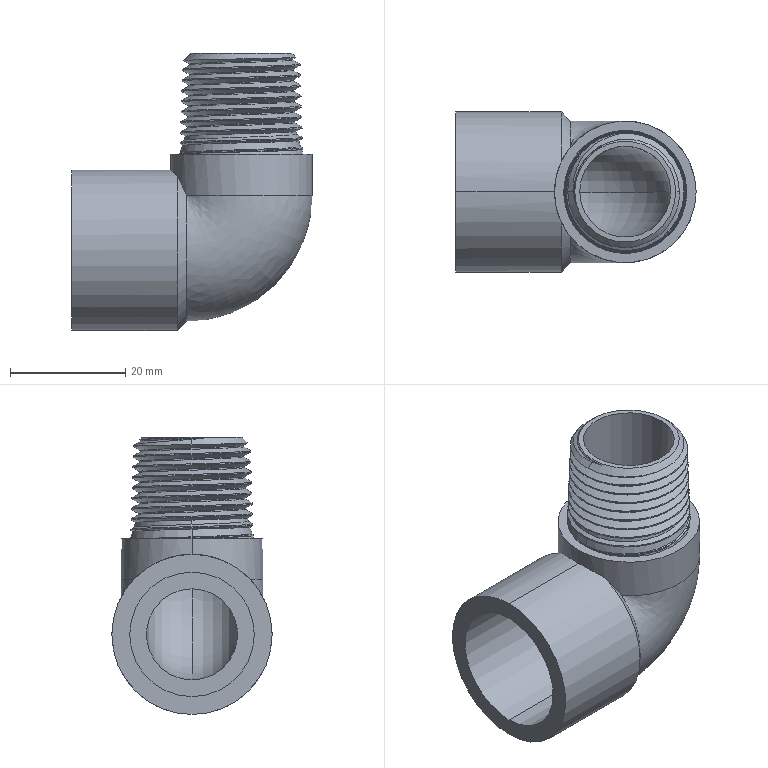Part | SolidWorks | 1 solid | 48 faces | box 41.648 x 27.781 x 48.022 mm | volume 12703 mm3 | cone 30 | cylinder 8 | spline 4 | plane 4 | torus 2 | commonest cylinder face diameters 15.799 x2 21.59 x2 24.559 x2 27.781 x2